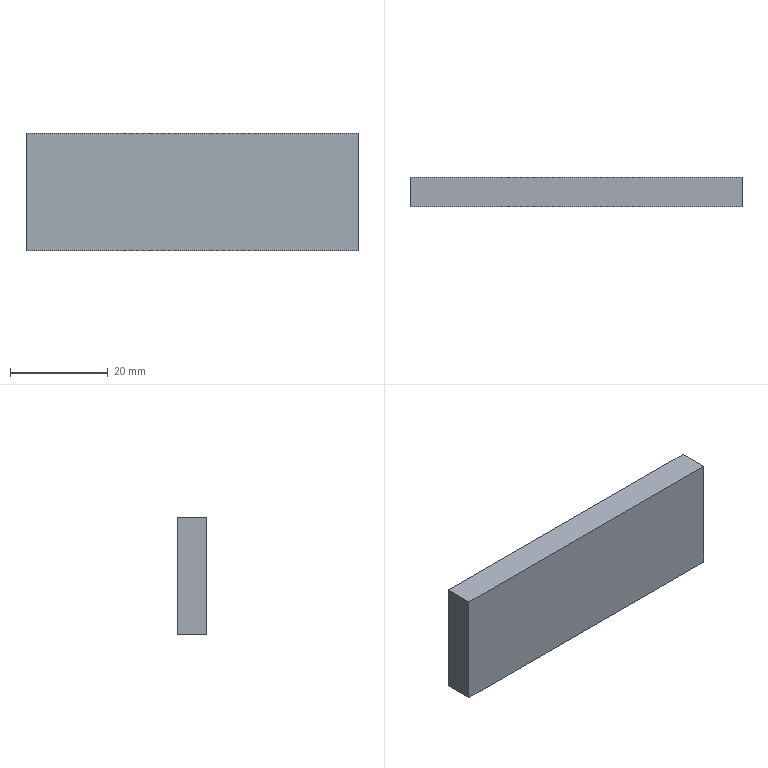Part | STEP file | 1005 | 1 solid | 6 faces | box 68 x 6 x 24 mm | volume 9792 mm3 | plane 6
STEP:
#1=CARTESIAN_POINT('',(0.,0.,0.));
#2=DIRECTION('',(0.,0.,1.));
#3=DIRECTION('',(1.,0.,0.));
#4=AXIS2_PLACEMENT_3D('',#1,#2,#3);
#5=CARTESIAN_POINT('',(34.,272.,35.));
#6=VERTEX_POINT('',#5);
#7=CARTESIAN_POINT('',(34.,272.,11.));
#8=VERTEX_POINT('',#7);
#9=CARTESIAN_POINT('',(34.,272.,0.));
#10=DIRECTION('',(0.,0.,-1.));
#11=VECTOR('',#10,1.);
#12=LINE('',#9,#11);
#13=CARTESIAN_POINT('',(0.,272.,0.));
#14=DIRECTION('',(0.,1.,0.));
#15=DIRECTION('',(0.,0.,1.));
#16=AXIS2_PLACEMENT_3D('',#13,#14,#15);
#17=PLANE('',#16);
#18=CARTESIAN_POINT('',(0.,34.));
#19=DIRECTION('',(-1.,0.));
#20=VECTOR('',#19,1.);
#21=LINE('',#18,#20);
#22=(GEOMETRIC_REPRESENTATION_CONTEXT(2)PARAMETRIC_REPRESENTATION_CONTEXT()REPRESENTATION_CONTEXT('',''));
#23=DEFINITIONAL_REPRESENTATION('',(#21),#22);
#24=PCURVE('',#17,#23);
#25=CARTESIAN_POINT('',(34.,272.,35.));
#26=DIRECTION('',(1.,0.,0.));
#27=DIRECTION('',(0.,0.,-1.));
#28=AXIS2_PLACEMENT_3D('',#25,#26,#27);
#29=PLANE('',#28);
#30=CARTESIAN_POINT('',(35.,0.));
#31=DIRECTION('',(1.,0.));
#32=VECTOR('',#31,1.);
#33=LINE('',#30,#32);
#34=(GEOMETRIC_REPRESENTATION_CONTEXT(2)PARAMETRIC_REPRESENTATION_CONTEXT()REPRESENTATION_CONTEXT('',''));
#35=DEFINITIONAL_REPRESENTATION('',(#33),#34);
#36=PCURVE('',#29,#35);
#37=SURFACE_CURVE('',#12,(#24,#36),.PCURVE_S1.);
#38=EDGE_CURVE('',#6,#8,#37,.T.);
#39=ORIENTED_EDGE('',*,*,#38,.T.);
#40=CARTESIAN_POINT('',(-34.,272.,11.));
#41=VERTEX_POINT('',#40);
#42=CARTESIAN_POINT('',(0.,272.,11.));
#43=DIRECTION('',(-1.,0.,0.));
#44=VECTOR('',#43,1.);
#45=LINE('',#42,#44);
#46=CARTESIAN_POINT('',(11.,0.));
#47=DIRECTION('',(0.,-1.));
#48=VECTOR('',#47,1.);
#49=LINE('',#46,#48);
#50=(GEOMETRIC_REPRESENTATION_CONTEXT(2)PARAMETRIC_REPRESENTATION_CONTEXT()REPRESENTATION_CONTEXT('',''));
#51=DEFINITIONAL_REPRESENTATION('',(#49),#50);
#52=PCURVE('',#17,#51);
#53=CARTESIAN_POINT('',(34.,272.,11.));
#54=DIRECTION('',(0.,0.,-1.));
#55=DIRECTION('',(-1.,0.,0.));
#56=AXIS2_PLACEMENT_3D('',#53,#54,#55);
#57=PLANE('',#56);
#58=CARTESIAN_POINT('',(34.,0.));
#59=DIRECTION('',(1.,0.));
#60=VECTOR('',#59,1.);
#61=LINE('',#58,#60);
#62=(GEOMETRIC_REPRESENTATION_CONTEXT(2)PARAMETRIC_REPRESENTATION_CONTEXT()REPRESENTATION_CONTEXT('',''));
#63=DEFINITIONAL_REPRESENTATION('',(#61),#62);
#64=PCURVE('',#57,#63);
#65=SURFACE_CURVE('',#45,(#52,#64),.PCURVE_S1.);
#66=EDGE_CURVE('',#8,#41,#65,.T.);
#67=ORIENTED_EDGE('',*,*,#66,.T.);
#68=CARTESIAN_POINT('',(-34.,272.,35.));
#69=VERTEX_POINT('',#68);
#70=CARTESIAN_POINT('',(-34.,272.,0.));
#71=DIRECTION('',(0.,0.,1.));
#72=VECTOR('',#71,1.);
#73=LINE('',#70,#72);
#74=CARTESIAN_POINT('',(0.,-34.));
#75=DIRECTION('',(1.,0.));
#76=VECTOR('',#75,1.);
#77=LINE('',#74,#76);
#78=(GEOMETRIC_REPRESENTATION_CONTEXT(2)PARAMETRIC_REPRESENTATION_CONTEXT()REPRESENTATION_CONTEXT('',''));
#79=DEFINITIONAL_REPRESENTATION('',(#77),#78);
#80=PCURVE('',#17,#79);
#81=CARTESIAN_POINT('',(-34.,272.,11.));
#82=DIRECTION('',(-1.,0.,0.));
#83=DIRECTION('',(0.,0.,1.));
#84=AXIS2_PLACEMENT_3D('',#81,#82,#83);
#85=PLANE('',#84);
#86=CARTESIAN_POINT('',(-11.,0.));
#87=DIRECTION('',(1.,0.));
#88=VECTOR('',#87,1.);
#89=LINE('',#86,#88);
#90=(GEOMETRIC_REPRESENTATION_CONTEXT(2)PARAMETRIC_REPRESENTATION_CONTEXT()REPRESENTATION_CONTEXT('',''));
#91=DEFINITIONAL_REPRESENTATION('',(#89),#90);
#92=PCURVE('',#85,#91);
#93=SURFACE_CURVE('',#73,(#80,#92),.PCURVE_S1.);
#94=EDGE_CURVE('',#41,#69,#93,.T.);
#95=ORIENTED_EDGE('',*,*,#94,.T.);
#96=CARTESIAN_POINT('',(0.,272.,35.));
#97=DIRECTION('',(1.,0.,0.));
#98=VECTOR('',#97,1.);
#99=LINE('',#96,#98);
#100=CARTESIAN_POINT('',(35.,0.));
#101=DIRECTION('',(0.,1.));
#102=VECTOR('',#101,1.);
#103=LINE('',#100,#102);
#104=(GEOMETRIC_REPRESENTATION_CONTEXT(2)PARAMETRIC_REPRESENTATION_CONTEXT()REPRESENTATION_CONTEXT('',''));
#105=DEFINITIONAL_REPRESENTATION('',(#103),#104);
#106=PCURVE('',#17,#105);
#107=CARTESIAN_POINT('',(-34.,272.,35.));
#108=DIRECTION('',(0.,0.,1.));
#109=DIRECTION('',(1.,0.,0.));
#110=AXIS2_PLACEMENT_3D('',#107,#108,#109);
#111=PLANE('',#110);
#112=CARTESIAN_POINT('',(34.,0.));
#113=DIRECTION('',(1.,0.));
#114=VECTOR('',#113,1.);
#115=LINE('',#112,#114);
#116=(GEOMETRIC_REPRESENTATION_CONTEXT(2)PARAMETRIC_REPRESENTATION_CONTEXT()REPRESENTATION_CONTEXT('',''));
#117=DEFINITIONAL_REPRESENTATION('',(#115),#116);
#118=PCURVE('',#111,#117);
#119=SURFACE_CURVE('',#99,(#106,#118),.PCURVE_S1.);
#120=EDGE_CURVE('',#69,#6,#119,.T.);
#121=ORIENTED_EDGE('',*,*,#120,.T.);
#122=EDGE_LOOP('',(#39,#67,#95,#121));
#123=FACE_BOUND('',#122,.T.);
#124=ADVANCED_FACE('',(#123),#17,.T.);
#125=CARTESIAN_POINT('',(-34.,266.,11.));
#126=VERTEX_POINT('',#125);
#127=CARTESIAN_POINT('',(-34.,272.,11.));
#128=DIRECTION('',(0.,1.,0.));
#129=VECTOR('',#128,1.);
#130=LINE('',#127,#129);
#131=CARTESIAN_POINT('',(68.,0.));
#132=DIRECTION('',(0.,1.));
#133=VECTOR('',#132,1.);
#134=LINE('',#131,#133);
#135=(GEOMETRIC_REPRESENTATION_CONTEXT(2)PARAMETRIC_REPRESENTATION_CONTEXT()REPRESENTATION_CONTEXT('',''));
#136=DEFINITIONAL_REPRESENTATION('',(#134),#135);
#137=PCURVE('',#57,#136);
#138=CARTESIAN_POINT('',(0.,0.));
#139=DIRECTION('',(0.,1.));
#140=VECTOR('',#139,1.);
#141=LINE('',#138,#140);
#142=(GEOMETRIC_REPRESENTATION_CONTEXT(2)PARAMETRIC_REPRESENTATION_CONTEXT()REPRESENTATION_CONTEXT('',''));
#143=DEFINITIONAL_REPRESENTATION('',(#141),#142);
#144=PCURVE('',#85,#143);
#145=SURFACE_CURVE('',#130,(#137,#144),.PCURVE_S1.);
#146=EDGE_CURVE('',#126,#41,#145,.T.);
#147=ORIENTED_EDGE('',*,*,#146,.T.);
#148=ORIENTED_EDGE('',*,*,#66,.F.);
#149=CARTESIAN_POINT('',(34.,266.,11.));
#150=VERTEX_POINT('',#149);
#151=CARTESIAN_POINT('',(34.,272.,11.));
#152=DIRECTION('',(0.,-1.,0.));
#153=VECTOR('',#152,1.);
#154=LINE('',#151,#153);
#155=CARTESIAN_POINT('',(0.,0.));
#156=DIRECTION('',(0.,-1.));
#157=VECTOR('',#156,1.);
#158=LINE('',#155,#157);
#159=(GEOMETRIC_REPRESENTATION_CONTEXT(2)PARAMETRIC_REPRESENTATION_CONTEXT()REPRESENTATION_CONTEXT('',''));
#160=DEFINITIONAL_REPRESENTATION('',(#158),#159);
#161=PCURVE('',#57,#160);
#162=CARTESIAN_POINT('',(24.,0.));
#163=DIRECTION('',(0.,-1.));
#164=VECTOR('',#163,1.);
#165=LINE('',#162,#164);
#166=(GEOMETRIC_REPRESENTATION_CONTEXT(2)PARAMETRIC_REPRESENTATION_CONTEXT()REPRESENTATION_CONTEXT('',''));
#167=DEFINITIONAL_REPRESENTATION('',(#165),#166);
#168=PCURVE('',#29,#167);
#169=SURFACE_CURVE('',#154,(#161,#168),.PCURVE_S1.);
#170=EDGE_CURVE('',#8,#150,#169,.T.);
#171=ORIENTED_EDGE('',*,*,#170,.T.);
#172=CARTESIAN_POINT('',(34.,266.,11.));
#173=DIRECTION('',(-1.,0.,0.));
#174=VECTOR('',#173,1.);
#175=LINE('',#172,#174);
#176=CARTESIAN_POINT('',(0.,-6.));
#177=DIRECTION('',(1.,0.));
#178=VECTOR('',#177,1.);
#179=LINE('',#176,#178);
#180=(GEOMETRIC_REPRESENTATION_CONTEXT(2)PARAMETRIC_REPRESENTATION_CONTEXT()REPRESENTATION_CONTEXT('',''));
#181=DEFINITIONAL_REPRESENTATION('',(#179),#180);
#182=PCURVE('',#57,#181);
#183=CARTESIAN_POINT('',(0.,266.,0.));
#184=DIRECTION('',(0.,1.,0.));
#185=DIRECTION('',(0.,0.,1.));
#186=AXIS2_PLACEMENT_3D('',#183,#184,#185);
#187=PLANE('',#186);
#188=CARTESIAN_POINT('',(11.,34.));
#189=DIRECTION('',(0.,-1.));
#190=VECTOR('',#189,1.);
#191=LINE('',#188,#190);
#192=(GEOMETRIC_REPRESENTATION_CONTEXT(2)PARAMETRIC_REPRESENTATION_CONTEXT()REPRESENTATION_CONTEXT('',''));
#193=DEFINITIONAL_REPRESENTATION('',(#191),#192);
#194=PCURVE('',#187,#193);
#195=SURFACE_CURVE('',#175,(#182,#194),.PCURVE_S1.);
#196=EDGE_CURVE('',#150,#126,#195,.T.);
#197=ORIENTED_EDGE('',*,*,#196,.T.);
#198=EDGE_LOOP('',(#147,#148,#171,#197));
#199=FACE_BOUND('',#198,.T.);
#200=ADVANCED_FACE('',(#199),#57,.T.);
#201=ORIENTED_EDGE('',*,*,#170,.F.);
#202=ORIENTED_EDGE('',*,*,#38,.F.);
#203=CARTESIAN_POINT('',(34.,266.,35.));
#204=VERTEX_POINT('',#203);
#205=CARTESIAN_POINT('',(34.,272.,35.));
#206=DIRECTION('',(0.,-1.,0.));
#207=VECTOR('',#206,1.);
#208=LINE('',#205,#207);
#209=CARTESIAN_POINT('',(0.,0.));
#210=DIRECTION('',(0.,-1.));
#211=VECTOR('',#210,1.);
#212=LINE('',#209,#211);
#213=(GEOMETRIC_REPRESENTATION_CONTEXT(2)PARAMETRIC_REPRESENTATION_CONTEXT()REPRESENTATION_CONTEXT('',''));
#214=DEFINITIONAL_REPRESENTATION('',(#212),#213);
#215=PCURVE('',#29,#214);
#216=CARTESIAN_POINT('',(68.,0.));
#217=DIRECTION('',(0.,-1.));
#218=VECTOR('',#217,1.);
#219=LINE('',#216,#218);
#220=(GEOMETRIC_REPRESENTATION_CONTEXT(2)PARAMETRIC_REPRESENTATION_CONTEXT()REPRESENTATION_CONTEXT('',''));
#221=DEFINITIONAL_REPRESENTATION('',(#219),#220);
#222=PCURVE('',#111,#221);
#223=SURFACE_CURVE('',#208,(#215,#222),.PCURVE_S1.);
#224=EDGE_CURVE('',#6,#204,#223,.T.);
#225=ORIENTED_EDGE('',*,*,#224,.T.);
#226=CARTESIAN_POINT('',(34.,266.,35.));
#227=DIRECTION('',(0.,0.,-1.));
#228=VECTOR('',#227,1.);
#229=LINE('',#226,#228);
#230=CARTESIAN_POINT('',(0.,-6.));
#231=DIRECTION('',(1.,0.));
#232=VECTOR('',#231,1.);
#233=LINE('',#230,#232);
#234=(GEOMETRIC_REPRESENTATION_CONTEXT(2)PARAMETRIC_REPRESENTATION_CONTEXT()REPRESENTATION_CONTEXT('',''));
#235=DEFINITIONAL_REPRESENTATION('',(#233),#234);
#236=PCURVE('',#29,#235);
#237=CARTESIAN_POINT('',(35.,34.));
#238=DIRECTION('',(-1.,0.));
#239=VECTOR('',#238,1.);
#240=LINE('',#237,#239);
#241=(GEOMETRIC_REPRESENTATION_CONTEXT(2)PARAMETRIC_REPRESENTATION_CONTEXT()REPRESENTATION_CONTEXT('',''));
#242=DEFINITIONAL_REPRESENTATION('',(#240),#241);
#243=PCURVE('',#187,#242);
#244=SURFACE_CURVE('',#229,(#236,#243),.PCURVE_S1.);
#245=EDGE_CURVE('',#204,#150,#244,.T.);
#246=ORIENTED_EDGE('',*,*,#245,.T.);
#247=EDGE_LOOP('',(#201,#202,#225,#246));
#248=FACE_BOUND('',#247,.T.);
#249=ADVANCED_FACE('',(#248),#29,.T.);
#250=ORIENTED_EDGE('',*,*,#224,.F.);
#251=ORIENTED_EDGE('',*,*,#120,.F.);
#252=CARTESIAN_POINT('',(-34.,266.,35.));
#253=VERTEX_POINT('',#252);
#254=CARTESIAN_POINT('',(-34.,272.,35.));
#255=DIRECTION('',(0.,-1.,0.));
#256=VECTOR('',#255,1.);
#257=LINE('',#254,#256);
#258=CARTESIAN_POINT('',(0.,0.));
#259=DIRECTION('',(0.,-1.));
#260=VECTOR('',#259,1.);
#261=LINE('',#258,#260);
#262=(GEOMETRIC_REPRESENTATION_CONTEXT(2)PARAMETRIC_REPRESENTATION_CONTEXT()REPRESENTATION_CONTEXT('',''));
#263=DEFINITIONAL_REPRESENTATION('',(#261),#262);
#264=PCURVE('',#111,#263);
#265=CARTESIAN_POINT('',(24.,0.));
#266=DIRECTION('',(0.,-1.));
#267=VECTOR('',#266,1.);
#268=LINE('',#265,#267);
#269=(GEOMETRIC_REPRESENTATION_CONTEXT(2)PARAMETRIC_REPRESENTATION_CONTEXT()REPRESENTATION_CONTEXT('',''));
#270=DEFINITIONAL_REPRESENTATION('',(#268),#269);
#271=PCURVE('',#85,#270);
#272=SURFACE_CURVE('',#257,(#264,#271),.PCURVE_S1.);
#273=EDGE_CURVE('',#69,#253,#272,.T.);
#274=ORIENTED_EDGE('',*,*,#273,.T.);
#275=CARTESIAN_POINT('',(-34.,266.,35.));
#276=DIRECTION('',(1.,0.,0.));
#277=VECTOR('',#276,1.);
#278=LINE('',#275,#277);
#279=CARTESIAN_POINT('',(0.,-6.));
#280=DIRECTION('',(1.,0.));
#281=VECTOR('',#280,1.);
#282=LINE('',#279,#281);
#283=(GEOMETRIC_REPRESENTATION_CONTEXT(2)PARAMETRIC_REPRESENTATION_CONTEXT()REPRESENTATION_CONTEXT('',''));
#284=DEFINITIONAL_REPRESENTATION('',(#282),#283);
#285=PCURVE('',#111,#284);
#286=CARTESIAN_POINT('',(35.,-34.));
#287=DIRECTION('',(0.,1.));
#288=VECTOR('',#287,1.);
#289=LINE('',#286,#288);
#290=(GEOMETRIC_REPRESENTATION_CONTEXT(2)PARAMETRIC_REPRESENTATION_CONTEXT()REPRESENTATION_CONTEXT('',''));
#291=DEFINITIONAL_REPRESENTATION('',(#289),#290);
#292=PCURVE('',#187,#291);
#293=SURFACE_CURVE('',#278,(#285,#292),.PCURVE_S1.);
#294=EDGE_CURVE('',#253,#204,#293,.T.);
#295=ORIENTED_EDGE('',*,*,#294,.T.);
#296=EDGE_LOOP('',(#250,#251,#274,#295));
#297=FACE_BOUND('',#296,.T.);
#298=ADVANCED_FACE('',(#297),#111,.T.);
#299=ORIENTED_EDGE('',*,*,#273,.F.);
#300=ORIENTED_EDGE('',*,*,#94,.F.);
#301=ORIENTED_EDGE('',*,*,#146,.F.);
#302=CARTESIAN_POINT('',(-34.,266.,11.));
#303=DIRECTION('',(0.,0.,1.));
#304=VECTOR('',#303,1.);
#305=LINE('',#302,#304);
#306=CARTESIAN_POINT('',(0.,-6.));
#307=DIRECTION('',(1.,0.));
#308=VECTOR('',#307,1.);
#309=LINE('',#306,#308);
#310=(GEOMETRIC_REPRESENTATION_CONTEXT(2)PARAMETRIC_REPRESENTATION_CONTEXT()REPRESENTATION_CONTEXT('',''));
#311=DEFINITIONAL_REPRESENTATION('',(#309),#310);
#312=PCURVE('',#85,#311);
#313=CARTESIAN_POINT('',(11.,-34.));
#314=DIRECTION('',(1.,0.));
#315=VECTOR('',#314,1.);
#316=LINE('',#313,#315);
#317=(GEOMETRIC_REPRESENTATION_CONTEXT(2)PARAMETRIC_REPRESENTATION_CONTEXT()REPRESENTATION_CONTEXT('',''));
#318=DEFINITIONAL_REPRESENTATION('',(#316),#317);
#319=PCURVE('',#187,#318);
#320=SURFACE_CURVE('',#305,(#312,#319),.PCURVE_S1.);
#321=EDGE_CURVE('',#126,#253,#320,.T.);
#322=ORIENTED_EDGE('',*,*,#321,.T.);
#323=EDGE_LOOP('',(#299,#300,#301,#322));
#324=FACE_BOUND('',#323,.T.);
#325=ADVANCED_FACE('',(#324),#85,.T.);
#326=ORIENTED_EDGE('',*,*,#294,.F.);
#327=ORIENTED_EDGE('',*,*,#321,.F.);
#328=ORIENTED_EDGE('',*,*,#196,.F.);
#329=ORIENTED_EDGE('',*,*,#245,.F.);
#330=EDGE_LOOP('',(#326,#327,#328,#329));
#331=FACE_BOUND('',#330,.T.);
#332=ADVANCED_FACE('',(#331),#187,.F.);
#333=CLOSED_SHELL('',(#124,#200,#249,#298,#325,#332));
#334=MANIFOLD_SOLID_BREP('',#333);
#335=(LENGTH_UNIT()NAMED_UNIT(*)SI_UNIT(.MILLI.,.METRE.));
#336=UNCERTAINTY_MEASURE_WITH_UNIT(LENGTH_MEASURE(0.0000001),#335,'','');
#337=(NAMED_UNIT(*)PLANE_ANGLE_UNIT()SI_UNIT($,.RADIAN.));
#338=(NAMED_UNIT(*)SI_UNIT($,.STERADIAN.)SOLID_ANGLE_UNIT());
#339=(GEOMETRIC_REPRESENTATION_CONTEXT(3)GLOBAL_UNCERTAINTY_ASSIGNED_CONTEXT((#336))GLOBAL_UNIT_ASSIGNED_CONTEXT((#335,#337,#338))REPRESENTATION_CONTEXT('',''));
#340=ADVANCED_BREP_SHAPE_REPRESENTATION('',(#4,#334),#339);